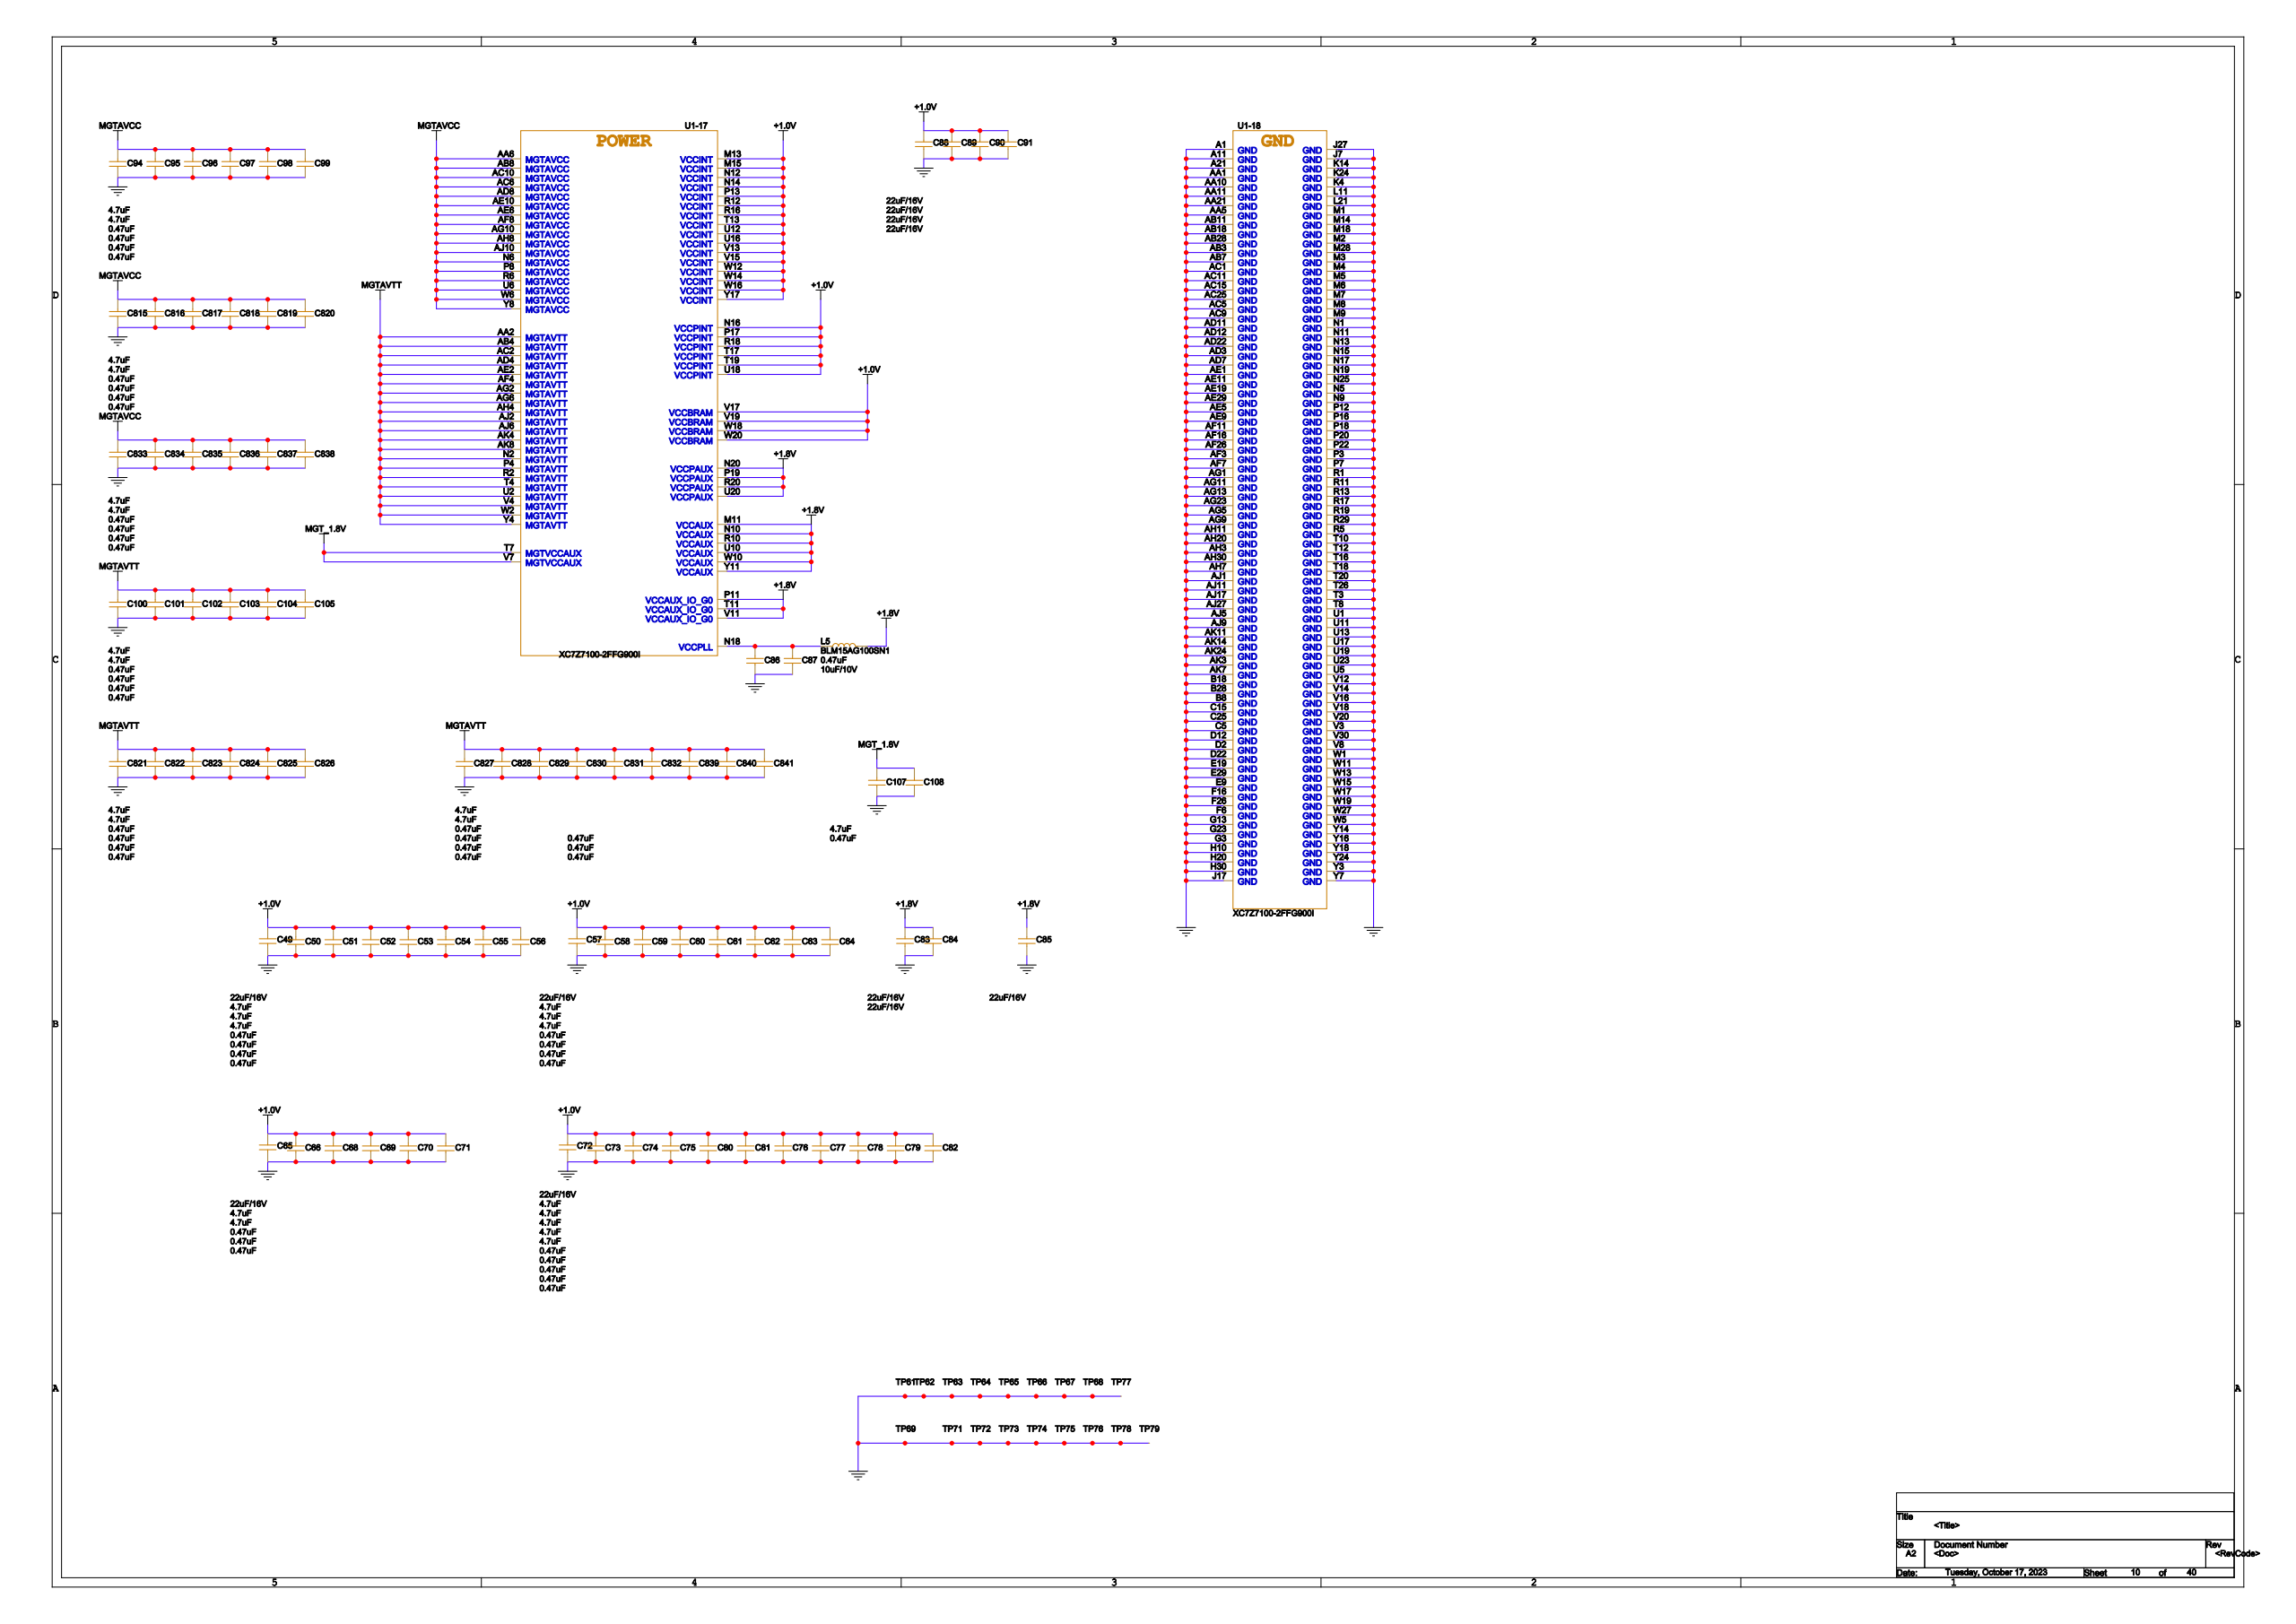Circuit board | Cadence Allegro | 1793 parts | 1223 nets | one sheet of the schematic
Parts on this sheet (reference | value | footprint):
C49 | 22uF/16V | C0603
C50 | 4.7uF | C0402
C51 | 4.7uF | C0402
C52 | 4.7uF | C0402
C53 | 0.47uF | C0402
C54 | 0.47uF | C0402
C55 | 0.47uF | C0402
C56 | 0.47uF | C0402
C57 | 22uF/16V | C0603
C58 | 4.7uF | C0402
C59 | 4.7uF | C0402
C60 | 4.7uF | C0402
C61 | 0.47uF | C0402
C62 | 0.47uF | C0402
C63 | 0.47uF | C0402
C64 | 0.47uF | C0402
C65 | 22uF/16V | C0603
C66 | 4.7uF | C0402
C68 | 4.7uF | C0402
C69 | 0.47uF | C0402
C70 | 0.47uF | C0402
C71 | 0.47uF | C0402
C72 | 22uF/16V | C0603
C73 | 4.7uF | C0402
C74 | 4.7uF | C0402
C75 | 4.7uF | C0402
C76 | 0.47uF | C0402
C77 | 0.47uF | C0402
C78 | 0.47uF | C0402
C79 | 0.47uF | C0402
C80 | 4.7uF | C0402
C81 | 4.7uF | C0402
C82 | 0.47uF | C0402
C83 | 22uF/16V | C0603
C84 | 22uF/16V | C0603
C85 | 22uF/16V | C0603
C86 | 0.47uF | C0402
C87 | 10uF/10V | C0402
C88 | 22uF/16V | C0603
C89 | 22uF/16V | C0603
C90 | 22uF/16V | C0603
C91 | 22uF/16V | C0603
C94 | 4.7uF | C0402
C95 | 4.7uF | C0402
C96 | 0.47uF | C0402
C97 | 0.47uF | C0402
C98 | 0.47uF | C0402
C99 | 0.47uF | C0402
C100 | 4.7uF | C0402
C101 | 4.7uF | C0402
C102 | 0.47uF | C0402
C103 | 0.47uF | C0402
C104 | 0.47uF | C0402
C105 | 0.47uF | C0402
C107 | 4.7uF | C0402
C108 | 0.47uF | C0402
C815 | 4.7uF | C0402
C816 | 4.7uF | C0402
C817 | 0.47uF | C0402
C818 | 0.47uF | C0402
C819 | 0.47uF | C0402
C820 | 0.47uF | C0402
C821 | 4.7uF | C0402
C822 | 4.7uF | C0402
C823 | 0.47uF | C0402
C824 | 0.47uF | C0402
C825 | 0.47uF | C0402
C826 | 0.47uF | C0402
C827 | 4.7uF | C0402
C828 | 4.7uF | C0402
C829 | 0.47uF | C0402
C830 | 0.47uF | C0402
C831 | 0.47uF | C0402
C832 | 0.47uF | C0402
C833 | 4.7uF | C0402
C834 | 4.7uF | C0402
C835 | 0.47uF | C0402
C836 | 0.47uF | C0402
C837 | 0.47uF | C0402
C838 | 0.47uF | C0402
C839 | 0.47uF | C0402
C840 | 0.47uF | C0402
C841 | 0.47uF | C0402
L5 | BLM15AG100SN1 | L0402
TP63 | TEST POINT A | Y300
TP64 | TEST POINT A | Y300
TP65 | TEST POINT A | Y300
TP66 | TEST POINT A | Y300
TP67 | TEST POINT A | Y300
TP68 | TEST POINT A | Y300
TP69 | TEST POINT A | Y300
TP71 | TEST POINT A | Y300
TP72 | TEST POINT A | Y300
TP73 | TEST POINT A | Y300
TP74 | TEST POINT A | Y300
TP75 | TEST POINT A | Y300
TP76 | TEST POINT A | Y300
TP77 | TEST POINT A | Y300
TP78 | TEST POINT A | Y300
TP79 | TEST POINT A | Y300
U1 | XC7Z7100-2FFG900I | FFG900
U5 | MT41J256M16 | FBGA-96
U11 | THGBMFG6C1LBAIL | VFBGA
Nets of these parts (net: part-pin ...):
GND: C49-2 C50-1 C51-1 C52-1 C53-1 C54-1 C55-1 C56-1 C57-2 C58-1 C59-1 C60-1 C61-1 C62-1 C63-1 C64-1 C65-2 C66-1 C68-1 C69-1 C70-1 C71-1 C72-2 C73-1 C74-1 C75-1 C76-1 C77-1 C78-1 C79-1 C80-1 C81-1 C82-1 C83-2 C84-2 C85-2 C86-1 C87-1 C88-2 C89-2 C90-2 C91-2 C94-1 C95-1 C96-1 C97-1 C98-1 C99-1 C100-1 C101-1 C102-1 C103-1 C104-1 C105-1 C107-1 C108-1 C815-1 C816-1 C817-1 C818-1 C819-1 C820-1 C821-1 C822-1 C823-1 C824-1 C825-1 C826-1 C827-1 C828-1 C829-1 C830-1 C831-1 C832-1 C833-1 C834-1 C835-1 C836-1 C837-1 C838-1 C839-1 C840-1 C841-1 TP63-1 TP64-1 TP65-1 TP66-1 TP67-1 TP68-1 TP69-1 TP71-1 TP72-1 TP73-1 TP74-1 TP75-1 TP76-1 TP77-1 TP78-1 TP79-1 U1-A1 U1-A11 U1-A21 U1-AA1 U1-AA5 U1-AA10 U1-AA11 U1-AA21 U1-AB3 U1-AB7 U1-AB11 U1-AB18 U1-AB28 U1-AC1 U1-AC5 U1-AC9 U1-AC11 U1-AC15 U1-AC25 U1-AD3 U1-AD7 U1-AD11 U1-AD12 U1-AD22 U1-AE1 U1-AE5 U1-AE9 U1-AE11 U1-AE19 U1-AE29 U1-AF3 U1-AF7 U1-AF11 U1-AF16 U1-AF26 U1-AG1 U1-AG5 U1-AG9 U1-AG11 U1-AG13 U1-AG23 U1-AH3 U1-AH7 U1-AH11 U1-AH20 U1-AH30 U1-AJ1 U1-AJ5 U1-AJ9 U1-AJ11 U1-AJ17 U1-AJ27 U1-AK3 U1-AK7 U1-AK11 U1-AK14 U1-AK24 U1-B8 U1-B18 U1-B28 U1-C5 U1-C15 U1-C25 U1-D2 U1-D12 U1-D22 U1-E9 U1-E19 U1-E29 U1-F6 U1-F16 U1-F26 U1-G3 U1-G13 U1-G23 U1-H10 U1-H20 U1-H30 U1-J7 U1-J17 U1-J27 U1-K4 U1-K14 U1-K24 U1-L11 U1-L21 U1-M1 U1-M2 U1-M3 U1-M4 U1-M5 U1-M6 U1-M7 U1-M8 U1-M9 U1-M14 U1-M18 U1-M28 U1-N1 U1-N5 U1-N9 U1-N11 U1-N13 U1-N15 U1-N17 U1-N19 U1-N25 U1-P3 U1-P7 U1-P12 U1-P16 U1-P18 U1-P20 U1-P22 U1-R1 U1-R5 U1-R11 U1-R13 U1-R17 U1-R19 U1-R29 U1-T3 U1-T8 U1-T10 U1-T12 U1-T16 U1-T18 U1-T20 U1-T26 U1-U1 U1-U5 U1-U11 U1-U13 U1-U17 U1-U19 U1-U23 U1-V3 U1-V8 U1-V12 U1-V14 U1-V16 U1-V18 U1-V20 U1-V30 U1-W1 U1-W5 U1-W11 U1-W13 U1-W15 U1-W17 U1-W19 U1-W27 U1-Y3 U1-Y7 U1-Y14 U1-Y16 U1-Y18 U1-Y24 U5-M1 U5-M9 U11-H10 U11-N2 U11-N5 U11-P4
MGTAVTT: C100-2 C101-2 C102-2 C103-2 C104-2 C105-2 C821-2 C822-2 C823-2 C824-2 C825-2 C826-2 C827-2 C828-2 C829-2 C830-2 C831-2 C832-2 C839-2 C840-2 C841-2 U1-AA2 U1-AB4 U1-AC2 U1-AD4 U1-AE2 U1-AF4 U1-AG2 U1-AG6 U1-AH4 U1-AJ2 U1-AJ6 U1-AK4 U1-AK8 U1-N2 U1-P4 U1-R2 U1-T4 U1-U2 U1-V4 U1-W2 U1-Y4
+1.0V: C49-1 C50-2 C51-2 C52-2 C53-2 C54-2 C55-2 C56-2 C57-1 C58-2 C59-2 C60-2 C61-2 C62-2 C63-2 C64-2 C65-1 C66-2 C68-2 C69-2 C70-2 C71-2 C72-1 C73-2 C74-2 C75-2 C76-2 C77-2 C78-2 C79-2 C80-2 C81-2 C82-2 C88-1 C89-1 C90-1 C91-1 U1-M13 U1-M15 U1-N12 U1-N14 U1-N16 U1-P13 U1-P17 U1-R12 U1-R16 U1-R18 U1-T13 U1-T17 U1-T19 U1-U12 U1-U16 U1-U18 U1-V13 U1-V15 U1-V17 U1-V19 U1-W12 U1-W14 U1-W16 U1-W18 U1-W20 U1-Y17
+1.8V: C83-1 C84-1 C85-1 L5-2 U1-M11 U1-N10 U1-N20 U1-P11 U1-P19 U1-R10 U1-R20 U1-T11 U1-U10 U1-U20 U1-V11 U1-W10 U1-Y11 U11-M4 U11-P3
MGTAVCC: C94-2 C95-2 C96-2 C97-2 C98-2 C99-2 C815-2 C816-2 C817-2 C818-2 C819-2 C820-2 C833-2 C834-2 C835-2 C836-2 C837-2 C838-2 U1-AA6 U1-AB8 U1-AC6 U1-AC10 U1-AD8 U1-AE6 U1-AE10 U1-AF8 U1-AG10 U1-AH8 U1-AJ10 U1-N6 U1-P8 U1-R6 U1-U6 U1-W6 U1-Y8
MGT_1.8V: C107-2 C108-2 U1-T7 U1-V7
N92594: C86-2 C87-2 L5-1 U1-N18